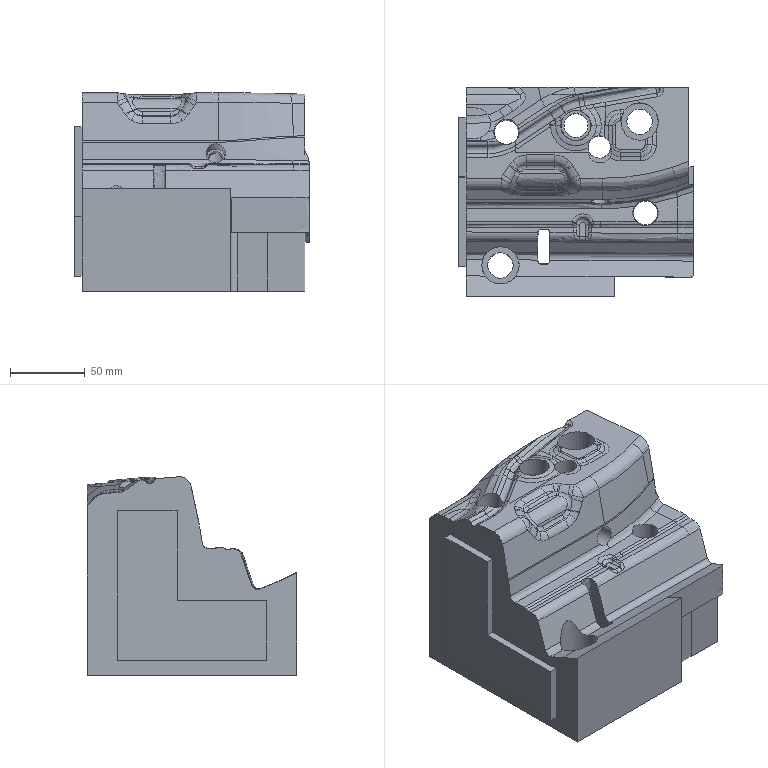Part | NX | features solid 2 | 1 solid | 264 faces | box 157 x 140.003 x 132.687 mm | volume 1902968 mm3 | spline 221 | plane 28 | cylinder 15 | commonest cylinder face diameters 17 x4 16 x3 10 x2 25 x2 13 x1 15 x1